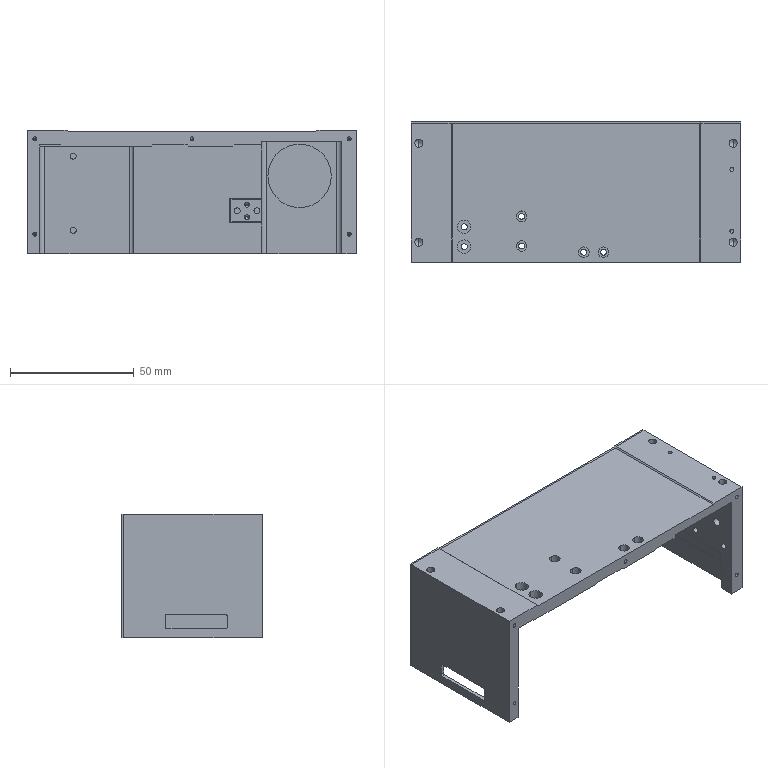Part | 3 solids | 284 faces | box 133 x 56.74 x 50 mm | volume 91541 mm3 | cylinder 151 | plane 87 | cone 46 | commonest cylinder face diameters 1.6 x32 2.4 x20 2 x18 4 x13 2.5 x12 4.3 x12